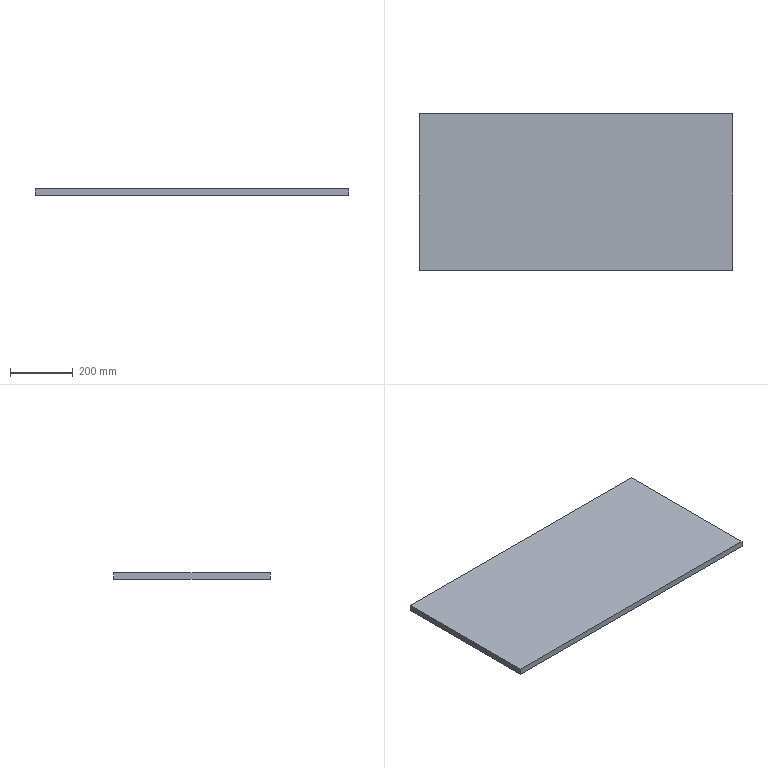Part | SolidWorks | features BaseBody 1 | 1 solid | 6 faces | box 1000 x 500 x 20 mm | volume 10000000 mm3 | plane 6
STEP:
#1=CARTESIAN_POINT('',(2587.963,1902.989,0.));
#2=VERTEX_POINT('',#1);
#3=CARTESIAN_POINT('',(2587.963,1902.989,20.));
#4=VERTEX_POINT('',#3);
#5=CARTESIAN_POINT('',(2587.963,1902.989,0.));
#6=DIRECTION('',(0.,0.,1.));
#7=VECTOR('',#6,1000.);
#8=LINE('',#5,#7);
#9=EDGE_CURVE('',#2,#4,#8,.T.);
#10=ORIENTED_EDGE('',*,*,#9,.F.);
#11=CARTESIAN_POINT('',(2587.963,1402.989,0.));
#12=VERTEX_POINT('',#11);
#13=CARTESIAN_POINT('',(2587.963,1402.989,0.));
#14=DIRECTION('',(0.,-1.,0.));
#15=VECTOR('',#14,1000.);
#16=LINE('',#13,#15);
#17=EDGE_CURVE('',#2,#12,#16,.T.);
#18=ORIENTED_EDGE('',*,*,#17,.T.);
#19=CARTESIAN_POINT('',(2587.963,1402.989,20.));
#20=VERTEX_POINT('',#19);
#21=CARTESIAN_POINT('',(2587.963,1402.989,20.));
#22=DIRECTION('',(0.,0.,-1.));
#23=VECTOR('',#22,1000.);
#24=LINE('',#21,#23);
#25=EDGE_CURVE('',#20,#12,#24,.T.);
#26=ORIENTED_EDGE('',*,*,#25,.F.);
#27=CARTESIAN_POINT('',(2587.963,1402.989,20.));
#28=DIRECTION('',(0.,-1.,0.));
#29=VECTOR('',#28,1000.);
#30=LINE('',#27,#29);
#31=EDGE_CURVE('',#4,#20,#30,.T.);
#32=ORIENTED_EDGE('',*,*,#31,.F.);
#33=EDGE_LOOP('',(#10,#18,#26,#32));
#34=FACE_OUTER_BOUND('',#33,.T.);
#35=CARTESIAN_POINT('',(2587.963,1402.989,20.));
#36=DIRECTION('',(1.,0.,0.));
#37=DIRECTION('',(0.,0.,-1.));
#38=AXIS2_PLACEMENT_3D('',#35,#36,#37);
#39=PLANE('',#38);
#40=ADVANCED_FACE('',(#34),#39,.F.);
#41=CARTESIAN_POINT('',(3587.963,1902.989,20.));
#42=VERTEX_POINT('',#41);
#43=CARTESIAN_POINT('',(3587.963,1902.989,0.));
#44=VERTEX_POINT('',#43);
#45=CARTESIAN_POINT('',(3587.963,1902.989,0.));
#46=DIRECTION('',(0.,0.,-1.));
#47=VECTOR('',#46,1000.);
#48=LINE('',#45,#47);
#49=EDGE_CURVE('',#42,#44,#48,.T.);
#50=ORIENTED_EDGE('',*,*,#49,.F.);
#51=CARTESIAN_POINT('',(3587.963,1402.989,20.));
#52=VERTEX_POINT('',#51);
#53=CARTESIAN_POINT('',(3587.963,1927.989,20.));
#54=DIRECTION('',(0.,1.,0.));
#55=VECTOR('',#54,1000.);
#56=LINE('',#53,#55);
#57=EDGE_CURVE('',#52,#42,#56,.T.);
#58=ORIENTED_EDGE('',*,*,#57,.F.);
#59=CARTESIAN_POINT('',(3587.963,1402.989,0.));
#60=VERTEX_POINT('',#59);
#61=CARTESIAN_POINT('',(3587.963,1402.989,20.));
#62=DIRECTION('',(0.,0.,-1.));
#63=VECTOR('',#62,1000.);
#64=LINE('',#61,#63);
#65=EDGE_CURVE('',#52,#60,#64,.T.);
#66=ORIENTED_EDGE('',*,*,#65,.T.);
#67=CARTESIAN_POINT('',(3587.963,1927.989,0.));
#68=DIRECTION('',(0.,1.,0.));
#69=VECTOR('',#68,1000.);
#70=LINE('',#67,#69);
#71=EDGE_CURVE('',#60,#44,#70,.T.);
#72=ORIENTED_EDGE('',*,*,#71,.T.);
#73=EDGE_LOOP('',(#50,#58,#66,#72));
#74=FACE_OUTER_BOUND('',#73,.T.);
#75=CARTESIAN_POINT('',(3587.963,1927.989,20.));
#76=DIRECTION('',(-1.,0.,0.));
#77=DIRECTION('',(0.,0.,1.));
#78=AXIS2_PLACEMENT_3D('',#75,#76,#77);
#79=PLANE('',#78);
#80=ADVANCED_FACE('',(#74),#79,.F.);
#81=CARTESIAN_POINT('',(2587.963,1902.989,20.));
#82=DIRECTION('',(1.,0.,0.));
#83=VECTOR('',#82,1000.);
#84=LINE('',#81,#83);
#85=EDGE_CURVE('',#4,#42,#84,.T.);
#86=ORIENTED_EDGE('',*,*,#85,.F.);
#87=ORIENTED_EDGE('',*,*,#31,.T.);
#88=CARTESIAN_POINT('',(3587.963,1402.989,20.));
#89=DIRECTION('',(1.,0.,0.));
#90=VECTOR('',#89,1000.);
#91=LINE('',#88,#90);
#92=EDGE_CURVE('',#20,#52,#91,.T.);
#93=ORIENTED_EDGE('',*,*,#92,.T.);
#94=ORIENTED_EDGE('',*,*,#57,.T.);
#95=EDGE_LOOP('',(#86,#87,#93,#94));
#96=FACE_OUTER_BOUND('',#95,.T.);
#97=CARTESIAN_POINT('',(0.,0.,20.));
#98=DIRECTION('',(0.,0.,-1.));
#99=DIRECTION('',(-1.,0.,0.));
#100=AXIS2_PLACEMENT_3D('',#97,#98,#99);
#101=PLANE('',#100);
#102=ADVANCED_FACE('',(#96),#101,.F.);
#103=ORIENTED_EDGE('',*,*,#17,.F.);
#104=CARTESIAN_POINT('',(2587.963,1902.989,0.));
#105=DIRECTION('',(-1.,0.,0.));
#106=VECTOR('',#105,1000.);
#107=LINE('',#104,#106);
#108=EDGE_CURVE('',#44,#2,#107,.T.);
#109=ORIENTED_EDGE('',*,*,#108,.F.);
#110=ORIENTED_EDGE('',*,*,#71,.F.);
#111=CARTESIAN_POINT('',(3587.963,1402.989,0.));
#112=DIRECTION('',(1.,0.,0.));
#113=VECTOR('',#112,1000.);
#114=LINE('',#111,#113);
#115=EDGE_CURVE('',#12,#60,#114,.T.);
#116=ORIENTED_EDGE('',*,*,#115,.F.);
#117=EDGE_LOOP('',(#103,#109,#110,#116));
#118=FACE_OUTER_BOUND('',#117,.T.);
#119=CARTESIAN_POINT('',(0.,0.,0.));
#120=DIRECTION('',(0.,0.,-1.));
#121=DIRECTION('',(-1.,0.,0.));
#122=AXIS2_PLACEMENT_3D('',#119,#120,#121);
#123=PLANE('',#122);
#124=ADVANCED_FACE('',(#118),#123,.T.);
#125=ORIENTED_EDGE('',*,*,#115,.T.);
#126=ORIENTED_EDGE('',*,*,#65,.F.);
#127=ORIENTED_EDGE('',*,*,#92,.F.);
#128=ORIENTED_EDGE('',*,*,#25,.T.);
#129=EDGE_LOOP('',(#125,#126,#127,#128));
#130=FACE_OUTER_BOUND('',#129,.T.);
#131=CARTESIAN_POINT('',(3587.963,1402.989,20.));
#132=DIRECTION('',(0.,1.,0.));
#133=DIRECTION('',(0.,0.,1.));
#134=AXIS2_PLACEMENT_3D('',#131,#132,#133);
#135=PLANE('',#134);
#136=ADVANCED_FACE('',(#130),#135,.F.);
#137=ORIENTED_EDGE('',*,*,#9,.T.);
#138=ORIENTED_EDGE('',*,*,#85,.T.);
#139=ORIENTED_EDGE('',*,*,#49,.T.);
#140=ORIENTED_EDGE('',*,*,#108,.T.);
#141=EDGE_LOOP('',(#137,#138,#139,#140));
#142=FACE_OUTER_BOUND('',#141,.T.);
#143=CARTESIAN_POINT('',(0.,1902.989,0.));
#144=DIRECTION('',(0.,1.,0.));
#145=DIRECTION('',(0.,0.,1.));
#146=AXIS2_PLACEMENT_3D('',#143,#144,#145);
#147=PLANE('',#146);
#148=ADVANCED_FACE('',(#142),#147,.T.);
#149=CLOSED_SHELL('',(#40,#80,#102,#124,#136,#148));
#150=MANIFOLD_SOLID_BREP('',#149);
#151=CARTESIAN_POINT('',(0.,0.,0.));
#152=DIRECTION('',(0.,0.,1.));
#153=DIRECTION('',(1.,0.,0.));
#154=AXIS2_PLACEMENT_3D('',#151,#152,#153);
#155=(LENGTH_UNIT()NAMED_UNIT(*)SI_UNIT(.MILLI.,.METRE.));
#156=UNCERTAINTY_MEASURE_WITH_UNIT(LENGTH_MEASURE(0.00001),#155,'','');
#157=(NAMED_UNIT(*)PLANE_ANGLE_UNIT()SI_UNIT($,.RADIAN.));
#158=(NAMED_UNIT(*)SI_UNIT($,.STERADIAN.)SOLID_ANGLE_UNIT());
#159=(GEOMETRIC_REPRESENTATION_CONTEXT(3)GLOBAL_UNCERTAINTY_ASSIGNED_CONTEXT((#156))GLOBAL_UNIT_ASSIGNED_CONTEXT((#155,#157,#158))REPRESENTATION_CONTEXT('',''));
#160=ADVANCED_BREP_SHAPE_REPRESENTATION('',(#150,#154),#159);